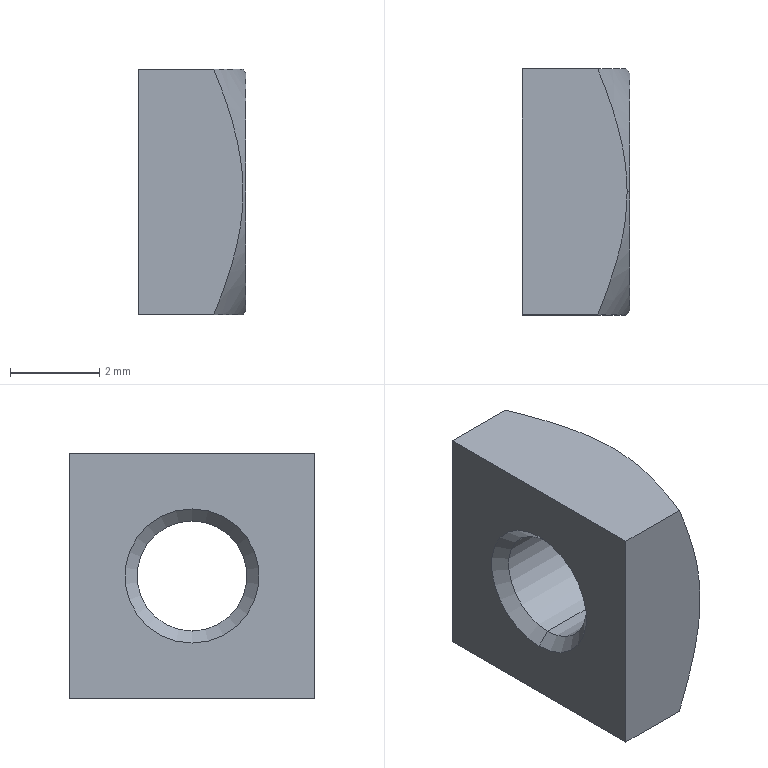Part | STEP file | Guide wheel mechanism revised.sldasm-Part-473 | 1 solid | 14 faces | box 2.4 x 5.5 x 5.5 mm | volume 58.875 mm3 | cone 6 | plane 6 | cylinder 2 | commonest cylinder face diameters 2.459 x2
STEP:
#1=CARTESIAN_POINT('',(2.129,0.,-1.229));
#2=VERTEX_POINT('',#1);
#3=CARTESIAN_POINT('',(2.129,0.,1.229));
#4=VERTEX_POINT('',#3);
#5=CARTESIAN_POINT('',(2.129,0.,0.));
#6=DIRECTION('',(-1.,0.,0.));
#7=DIRECTION('',(0.,0.,1.));
#8=AXIS2_PLACEMENT_3D('',#5,#6,#7);
#9=CIRCLE('',#8,1.229);
#10=EDGE_CURVE('',#2,#4,#9,.T.);
#11=ORIENTED_EDGE('',*,*,#10,.T.);
#12=CARTESIAN_POINT('',(2.4,0.,1.5));
#13=VERTEX_POINT('',#12);
#14=CARTESIAN_POINT('',(2.4,0.,1.5));
#15=DIRECTION('',(0.7071,0.,0.7071));
#16=VECTOR('',#15,1000.);
#17=LINE('',#14,#16);
#18=EDGE_CURVE('',#4,#13,#17,.T.);
#19=ORIENTED_EDGE('',*,*,#18,.T.);
#20=CARTESIAN_POINT('',(2.4,0.,-1.5));
#21=VERTEX_POINT('',#20);
#22=CARTESIAN_POINT('',(2.4,0.,0.));
#23=DIRECTION('',(-1.,0.,0.));
#24=DIRECTION('',(0.,0.,1.));
#25=AXIS2_PLACEMENT_3D('',#22,#23,#24);
#26=CIRCLE('',#25,1.5);
#27=EDGE_CURVE('',#21,#13,#26,.T.);
#28=ORIENTED_EDGE('',*,*,#27,.F.);
#29=CARTESIAN_POINT('',(2.4,0.,-1.5));
#30=DIRECTION('',(0.7071,0.,-0.7071));
#31=VECTOR('',#30,1000.);
#32=LINE('',#29,#31);
#33=EDGE_CURVE('',#2,#21,#32,.T.);
#34=ORIENTED_EDGE('',*,*,#33,.F.);
#35=EDGE_LOOP('',(#11,#19,#28,#34));
#36=FACE_OUTER_BOUND('',#35,.T.);
#37=CARTESIAN_POINT('',(2.4,0.,0.));
#38=DIRECTION('',(1.,0.,0.));
#39=DIRECTION('',(0.,0.,-1.));
#40=AXIS2_PLACEMENT_3D('',#37,#38,#39);
#41=CONICAL_SURFACE('',#40,1.5,0.7854);
#42=ADVANCED_FACE('',(#36),#41,.F.);
#43=ORIENTED_EDGE('',*,*,#10,.F.);
#44=CARTESIAN_POINT('',(0.2705,0.,-1.229));
#45=VERTEX_POINT('',#44);
#46=CARTESIAN_POINT('',(2.4,0.,-1.229));
#47=DIRECTION('',(-1.,0.,0.));
#48=VECTOR('',#47,1000.);
#49=LINE('',#46,#48);
#50=EDGE_CURVE('',#2,#45,#49,.T.);
#51=ORIENTED_EDGE('',*,*,#50,.T.);
#52=CARTESIAN_POINT('',(0.2705,0.,1.229));
#53=VERTEX_POINT('',#52);
#54=CARTESIAN_POINT('',(0.2705,0.,0.));
#55=DIRECTION('',(-1.,0.,0.));
#56=DIRECTION('',(0.,0.,1.));
#57=AXIS2_PLACEMENT_3D('',#54,#55,#56);
#58=CIRCLE('',#57,1.229);
#59=EDGE_CURVE('',#45,#53,#58,.T.);
#60=ORIENTED_EDGE('',*,*,#59,.T.);
#61=CARTESIAN_POINT('',(2.4,0.,1.229));
#62=DIRECTION('',(-1.,0.,0.));
#63=VECTOR('',#62,1000.);
#64=LINE('',#61,#63);
#65=EDGE_CURVE('',#4,#53,#64,.T.);
#66=ORIENTED_EDGE('',*,*,#65,.F.);
#67=EDGE_LOOP('',(#43,#51,#60,#66));
#68=FACE_OUTER_BOUND('',#67,.T.);
#69=CARTESIAN_POINT('',(2.4,0.,0.));
#70=DIRECTION('',(-1.,0.,0.));
#71=DIRECTION('',(0.,0.,1.));
#72=AXIS2_PLACEMENT_3D('',#69,#70,#71);
#73=CYLINDRICAL_SURFACE('',#72,1.229);
#74=ADVANCED_FACE('',(#68),#73,.F.);
#75=ORIENTED_EDGE('',*,*,#59,.F.);
#76=CARTESIAN_POINT('',(0.,0.,-1.5));
#77=VERTEX_POINT('',#76);
#78=CARTESIAN_POINT('',(0.2705,0.,-1.229));
#79=DIRECTION('',(-0.7071,0.,-0.7071));
#80=VECTOR('',#79,1000.);
#81=LINE('',#78,#80);
#82=EDGE_CURVE('',#45,#77,#81,.T.);
#83=ORIENTED_EDGE('',*,*,#82,.T.);
#84=CARTESIAN_POINT('',(0.,0.,1.5));
#85=VERTEX_POINT('',#84);
#86=CARTESIAN_POINT('',(0.,0.,0.));
#87=DIRECTION('',(-1.,0.,0.));
#88=DIRECTION('',(0.,0.,1.));
#89=AXIS2_PLACEMENT_3D('',#86,#87,#88);
#90=CIRCLE('',#89,1.5);
#91=EDGE_CURVE('',#77,#85,#90,.T.);
#92=ORIENTED_EDGE('',*,*,#91,.T.);
#93=CARTESIAN_POINT('',(0.2705,0.,1.229));
#94=DIRECTION('',(-0.7071,0.,0.7071));
#95=VECTOR('',#94,1000.);
#96=LINE('',#93,#95);
#97=EDGE_CURVE('',#53,#85,#96,.T.);
#98=ORIENTED_EDGE('',*,*,#97,.F.);
#99=EDGE_LOOP('',(#75,#83,#92,#98));
#100=FACE_OUTER_BOUND('',#99,.T.);
#101=CARTESIAN_POINT('',(0.2705,0.,0.));
#102=DIRECTION('',(-1.,0.,0.));
#103=DIRECTION('',(0.,0.,1.));
#104=AXIS2_PLACEMENT_3D('',#101,#102,#103);
#105=CONICAL_SURFACE('',#104,1.229,0.7854);
#106=ADVANCED_FACE('',(#100),#105,.F.);
#107=CARTESIAN_POINT('',(2.4,0.,2.65));
#108=VERTEX_POINT('',#107);
#109=CARTESIAN_POINT('',(2.4,0.,-2.65));
#110=VERTEX_POINT('',#109);
#111=CARTESIAN_POINT('',(2.4,0.,0.));
#112=DIRECTION('',(-1.,0.,0.));
#113=DIRECTION('',(0.,0.,1.));
#114=AXIS2_PLACEMENT_3D('',#111,#112,#113);
#115=CIRCLE('',#114,2.65);
#116=EDGE_CURVE('',#108,#110,#115,.T.);
#117=ORIENTED_EDGE('',*,*,#116,.T.);
#118=CARTESIAN_POINT('',(2.342,0.,-2.75));
#119=VERTEX_POINT('',#118);
#120=CARTESIAN_POINT('',(2.4,0.,-2.65));
#121=DIRECTION('',(-0.5,0.,-0.866));
#122=VECTOR('',#121,1000.);
#123=LINE('',#120,#122);
#124=EDGE_CURVE('',#110,#119,#123,.T.);
#125=ORIENTED_EDGE('',*,*,#124,.T.);
#126=CARTESIAN_POINT('',(1.685,2.75,-2.75));
#127=VERTEX_POINT('',#126);
#128=CARTESIAN_POINT('',(2.342,0.,-2.75));
#129=CARTESIAN_POINT('',(2.342,0.4777,-2.75));
#130=CARTESIAN_POINT('',(2.268,0.9433,-2.75));
#131=CARTESIAN_POINT('',(2.028,1.859,-2.75));
#132=CARTESIAN_POINT('',(1.864,2.311,-2.75));
#133=CARTESIAN_POINT('',(1.685,2.75,-2.75));
#134=B_SPLINE_CURVE_WITH_KNOTS('',3,(#128,#129,#130,#131,#132,#133),.UNSPECIFIED.,.F.,.F.,(4,2,4),(0.00576,0.007192,0.008623),.UNSPECIFIED.);
#135=EDGE_CURVE('',#119,#127,#134,.T.);
#136=ORIENTED_EDGE('',*,*,#135,.T.);
#137=CARTESIAN_POINT('',(1.685,2.75,2.75));
#138=VERTEX_POINT('',#137);
#139=CARTESIAN_POINT('',(1.685,2.75,-2.75));
#140=CARTESIAN_POINT('',(1.864,2.75,-2.309));
#141=CARTESIAN_POINT('',(2.028,2.75,-1.859));
#142=CARTESIAN_POINT('',(2.209,2.75,-1.17));
#143=CARTESIAN_POINT('',(2.258,2.75,-0.9383));
#144=CARTESIAN_POINT('',(2.325,2.75,-0.4681));
#145=CARTESIAN_POINT('',(2.343,2.75,-0.2274));
#146=CARTESIAN_POINT('',(2.341,2.75,0.4863));
#147=CARTESIAN_POINT('',(2.267,2.75,0.95));
#148=CARTESIAN_POINT('',(2.027,2.75,1.863));
#149=CARTESIAN_POINT('',(1.863,2.75,2.312));
#150=CARTESIAN_POINT('',(1.685,2.75,2.75));
#151=B_SPLINE_CURVE_WITH_KNOTS('',3,(#139,#140,#141,#142,#143,#144,#145,#146,#147,#148,#149,#150),.UNSPECIFIED.,.F.,.F.,(4,2,2,2,2,4),(0.002918,0.004344,0.005057,0.00577,0.007197,0.008623),.UNSPECIFIED.);
#152=EDGE_CURVE('',#127,#138,#151,.T.);
#153=ORIENTED_EDGE('',*,*,#152,.T.);
#154=CARTESIAN_POINT('',(2.342,0.,2.75));
#155=VERTEX_POINT('',#154);
#156=CARTESIAN_POINT('',(1.685,2.75,2.75));
#157=CARTESIAN_POINT('',(1.864,2.311,2.75));
#158=CARTESIAN_POINT('',(2.028,1.859,2.75));
#159=CARTESIAN_POINT('',(2.268,0.9433,2.75));
#160=CARTESIAN_POINT('',(2.342,0.4777,2.75));
#161=CARTESIAN_POINT('',(2.342,0.,2.75));
#162=B_SPLINE_CURVE_WITH_KNOTS('',3,(#156,#157,#158,#159,#160,#161),.UNSPECIFIED.,.F.,.F.,(4,2,4),(0.007165,0.008584,0.01),.UNSPECIFIED.);
#163=EDGE_CURVE('',#138,#155,#162,.T.);
#164=ORIENTED_EDGE('',*,*,#163,.T.);
#165=CARTESIAN_POINT('',(2.4,0.,2.65));
#166=DIRECTION('',(-0.5,0.,0.866));
#167=VECTOR('',#166,1000.);
#168=LINE('',#165,#167);
#169=EDGE_CURVE('',#108,#155,#168,.T.);
#170=ORIENTED_EDGE('',*,*,#169,.F.);
#171=EDGE_LOOP('',(#117,#125,#136,#153,#164,#170));
#172=FACE_OUTER_BOUND('',#171,.T.);
#173=CARTESIAN_POINT('',(2.4,0.,0.));
#174=DIRECTION('',(-1.,0.,0.));
#175=DIRECTION('',(0.,0.,1.));
#176=AXIS2_PLACEMENT_3D('',#173,#174,#175);
#177=CONICAL_SURFACE('',#176,2.65,1.047);
#178=ADVANCED_FACE('',(#172),#177,.T.);
#179=ORIENTED_EDGE('',*,*,#116,.F.);
#180=CARTESIAN_POINT('',(2.4,0.,0.));
#181=DIRECTION('',(-1.,0.,0.));
#182=DIRECTION('',(0.,0.,1.));
#183=AXIS2_PLACEMENT_3D('',#180,#181,#182);
#184=CIRCLE('',#183,2.65);
#185=EDGE_CURVE('',#110,#108,#184,.T.);
#186=ORIENTED_EDGE('',*,*,#185,.F.);
#187=EDGE_LOOP('',(#179,#186));
#188=FACE_OUTER_BOUND('',#187,.T.);
#189=ORIENTED_EDGE('',*,*,#27,.T.);
#190=CARTESIAN_POINT('',(2.4,0.,0.));
#191=DIRECTION('',(-1.,0.,0.));
#192=DIRECTION('',(0.,0.,1.));
#193=AXIS2_PLACEMENT_3D('',#190,#191,#192);
#194=CIRCLE('',#193,1.5);
#195=EDGE_CURVE('',#13,#21,#194,.T.);
#196=ORIENTED_EDGE('',*,*,#195,.T.);
#197=EDGE_LOOP('',(#189,#196));
#198=FACE_BOUND('',#197,.T.);
#199=CARTESIAN_POINT('',(2.4,2.65,0.));
#200=DIRECTION('',(-1.,0.,0.));
#201=DIRECTION('',(0.,0.,1.));
#202=AXIS2_PLACEMENT_3D('',#199,#200,#201);
#203=PLANE('',#202);
#204=ADVANCED_FACE('',(#188,#198),#203,.F.);
#205=CARTESIAN_POINT('',(0.,2.75,2.75));
#206=VERTEX_POINT('',#205);
#207=CARTESIAN_POINT('',(0.,-2.75,2.75));
#208=VERTEX_POINT('',#207);
#209=CARTESIAN_POINT('',(0.,2.75,2.75));
#210=DIRECTION('',(0.,-1.,0.));
#211=VECTOR('',#210,1000.);
#212=LINE('',#209,#211);
#213=EDGE_CURVE('',#206,#208,#212,.T.);
#214=ORIENTED_EDGE('',*,*,#213,.F.);
#215=CARTESIAN_POINT('',(0.,2.75,-2.75));
#216=VERTEX_POINT('',#215);
#217=CARTESIAN_POINT('',(0.,2.75,-2.75));
#218=DIRECTION('',(0.,0.,1.));
#219=VECTOR('',#218,1000.);
#220=LINE('',#217,#219);
#221=EDGE_CURVE('',#216,#206,#220,.T.);
#222=ORIENTED_EDGE('',*,*,#221,.F.);
#223=CARTESIAN_POINT('',(0.,-2.75,-2.75));
#224=VERTEX_POINT('',#223);
#225=CARTESIAN_POINT('',(0.,-2.75,-2.75));
#226=DIRECTION('',(0.,1.,0.));
#227=VECTOR('',#226,1000.);
#228=LINE('',#225,#227);
#229=EDGE_CURVE('',#224,#216,#228,.T.);
#230=ORIENTED_EDGE('',*,*,#229,.F.);
#231=CARTESIAN_POINT('',(0.,-2.75,2.75));
#232=DIRECTION('',(0.,0.,-1.));
#233=VECTOR('',#232,1000.);
#234=LINE('',#231,#233);
#235=EDGE_CURVE('',#208,#224,#234,.T.);
#236=ORIENTED_EDGE('',*,*,#235,.F.);
#237=EDGE_LOOP('',(#214,#222,#230,#236));
#238=FACE_OUTER_BOUND('',#237,.T.);
#239=CARTESIAN_POINT('',(0.,0.,0.));
#240=DIRECTION('',(-1.,0.,0.));
#241=DIRECTION('',(0.,0.,1.));
#242=AXIS2_PLACEMENT_3D('',#239,#240,#241);
#243=CIRCLE('',#242,1.5);
#244=EDGE_CURVE('',#85,#77,#243,.T.);
#245=ORIENTED_EDGE('',*,*,#244,.F.);
#246=ORIENTED_EDGE('',*,*,#91,.F.);
#247=EDGE_LOOP('',(#245,#246));
#248=FACE_BOUND('',#247,.T.);
#249=CARTESIAN_POINT('',(0.,0.,0.));
#250=DIRECTION('',(1.,0.,0.));
#251=DIRECTION('',(0.,0.,-1.));
#252=AXIS2_PLACEMENT_3D('',#249,#250,#251);
#253=PLANE('',#252);
#254=ADVANCED_FACE('',(#238,#248),#253,.F.);
#255=ORIENTED_EDGE('',*,*,#124,.F.);
#256=ORIENTED_EDGE('',*,*,#185,.T.);
#257=ORIENTED_EDGE('',*,*,#169,.T.);
#258=CARTESIAN_POINT('',(1.685,-2.75,2.75));
#259=VERTEX_POINT('',#258);
#260=CARTESIAN_POINT('',(2.342,0.,2.75));
#261=CARTESIAN_POINT('',(2.342,-0.2371,2.75));
#262=CARTESIAN_POINT('',(2.324,-0.4768,2.75));
#263=CARTESIAN_POINT('',(2.256,-0.9452,2.75));
#264=CARTESIAN_POINT('',(2.207,-1.176,2.75));
#265=CARTESIAN_POINT('',(2.027,-1.862,2.75));
#266=CARTESIAN_POINT('',(1.864,-2.311,2.75));
#267=CARTESIAN_POINT('',(1.685,-2.75,2.75));
#268=B_SPLINE_CURVE_WITH_KNOTS('',3,(#260,#261,#262,#263,#264,#265,#266,#267),.UNSPECIFIED.,.F.,.F.,(4,2,2,4),(0.01,0.01071,0.01141,0.01282),.UNSPECIFIED.);
#269=EDGE_CURVE('',#155,#259,#268,.T.);
#270=ORIENTED_EDGE('',*,*,#269,.T.);
#271=CARTESIAN_POINT('',(1.685,-2.75,-2.75));
#272=VERTEX_POINT('',#271);
#273=CARTESIAN_POINT('',(1.685,-2.75,2.75));
#274=CARTESIAN_POINT('',(1.863,-2.75,2.312));
#275=CARTESIAN_POINT('',(2.027,-2.75,1.863));
#276=CARTESIAN_POINT('',(2.267,-2.75,0.95));
#277=CARTESIAN_POINT('',(2.341,-2.75,0.4863));
#278=CARTESIAN_POINT('',(2.343,-2.75,-0.2274));
#279=CARTESIAN_POINT('',(2.325,-2.75,-0.4681));
#280=CARTESIAN_POINT('',(2.258,-2.75,-0.9383));
#281=CARTESIAN_POINT('',(2.209,-2.75,-1.17));
#282=CARTESIAN_POINT('',(2.028,-2.75,-1.859));
#283=CARTESIAN_POINT('',(1.864,-2.75,-2.309));
#284=CARTESIAN_POINT('',(1.685,-2.75,-2.75));
#285=B_SPLINE_CURVE_WITH_KNOTS('',3,(#273,#274,#275,#276,#277,#278,#279,#280,#281,#282,#283,#284),.UNSPECIFIED.,.F.,.F.,(4,2,2,2,2,4),(0.007165,0.008579,0.009994,0.0107,0.01141,0.01282),.UNSPECIFIED.);
#286=EDGE_CURVE('',#259,#272,#285,.T.);
#287=ORIENTED_EDGE('',*,*,#286,.T.);
#288=CARTESIAN_POINT('',(1.685,-2.75,-2.75));
#289=CARTESIAN_POINT('',(1.864,-2.311,-2.75));
#290=CARTESIAN_POINT('',(2.027,-1.862,-2.75));
#291=CARTESIAN_POINT('',(2.207,-1.176,-2.75));
#292=CARTESIAN_POINT('',(2.256,-0.9452,-2.75));
#293=CARTESIAN_POINT('',(2.324,-0.4768,-2.75));
#294=CARTESIAN_POINT('',(2.342,-0.2371,-2.75));
#295=CARTESIAN_POINT('',(2.342,0.,-2.75));
#296=B_SPLINE_CURVE_WITH_KNOTS('',3,(#288,#289,#290,#291,#292,#293,#294,#295),.UNSPECIFIED.,.F.,.F.,(4,2,2,4),(0.002918,0.004339,0.005049,0.00576),.UNSPECIFIED.);
#297=EDGE_CURVE('',#272,#119,#296,.T.);
#298=ORIENTED_EDGE('',*,*,#297,.T.);
#299=EDGE_LOOP('',(#255,#256,#257,#270,#287,#298));
#300=FACE_OUTER_BOUND('',#299,.T.);
#301=CARTESIAN_POINT('',(2.4,0.,0.));
#302=DIRECTION('',(-1.,0.,0.));
#303=DIRECTION('',(0.,0.,1.));
#304=AXIS2_PLACEMENT_3D('',#301,#302,#303);
#305=CONICAL_SURFACE('',#304,2.65,1.047);
#306=ADVANCED_FACE('',(#300),#305,.T.);
#307=CARTESIAN_POINT('',(6.,2.75,-2.75));
#308=DIRECTION('',(-1.,0.,0.));
#309=VECTOR('',#308,1000.);
#310=LINE('',#307,#309);
#311=EDGE_CURVE('',#127,#216,#310,.T.);
#312=ORIENTED_EDGE('',*,*,#311,.T.);
#313=ORIENTED_EDGE('',*,*,#221,.T.);
#314=CARTESIAN_POINT('',(6.,2.75,2.75));
#315=DIRECTION('',(-1.,0.,0.));
#316=VECTOR('',#315,1000.);
#317=LINE('',#314,#316);
#318=EDGE_CURVE('',#138,#206,#317,.T.);
#319=ORIENTED_EDGE('',*,*,#318,.F.);
#320=ORIENTED_EDGE('',*,*,#152,.F.);
#321=EDGE_LOOP('',(#312,#313,#319,#320));
#322=FACE_OUTER_BOUND('',#321,.T.);
#323=CARTESIAN_POINT('',(6.,2.75,-2.75));
#324=DIRECTION('',(0.,-1.,0.));
#325=DIRECTION('',(0.,0.,-1.));
#326=AXIS2_PLACEMENT_3D('',#323,#324,#325);
#327=PLANE('',#326);
#328=ADVANCED_FACE('',(#322),#327,.F.);
#329=ORIENTED_EDGE('',*,*,#318,.T.);
#330=ORIENTED_EDGE('',*,*,#213,.T.);
#331=CARTESIAN_POINT('',(6.,-2.75,2.75));
#332=DIRECTION('',(-1.,0.,0.));
#333=VECTOR('',#332,1000.);
#334=LINE('',#331,#333);
#335=EDGE_CURVE('',#259,#208,#334,.T.);
#336=ORIENTED_EDGE('',*,*,#335,.F.);
#337=ORIENTED_EDGE('',*,*,#269,.F.);
#338=ORIENTED_EDGE('',*,*,#163,.F.);
#339=EDGE_LOOP('',(#329,#330,#336,#337,#338));
#340=FACE_OUTER_BOUND('',#339,.T.);
#341=CARTESIAN_POINT('',(6.,2.75,2.75));
#342=DIRECTION('',(0.,0.,-1.));
#343=DIRECTION('',(-1.,0.,0.));
#344=AXIS2_PLACEMENT_3D('',#341,#342,#343);
#345=PLANE('',#344);
#346=ADVANCED_FACE('',(#340),#345,.F.);
#347=ORIENTED_EDGE('',*,*,#335,.T.);
#348=ORIENTED_EDGE('',*,*,#235,.T.);
#349=CARTESIAN_POINT('',(6.,-2.75,-2.75));
#350=DIRECTION('',(-1.,0.,0.));
#351=VECTOR('',#350,1000.);
#352=LINE('',#349,#351);
#353=EDGE_CURVE('',#272,#224,#352,.T.);
#354=ORIENTED_EDGE('',*,*,#353,.F.);
#355=ORIENTED_EDGE('',*,*,#286,.F.);
#356=EDGE_LOOP('',(#347,#348,#354,#355));
#357=FACE_OUTER_BOUND('',#356,.T.);
#358=CARTESIAN_POINT('',(6.,-2.75,2.75));
#359=DIRECTION('',(0.,1.,0.));
#360=DIRECTION('',(0.,0.,1.));
#361=AXIS2_PLACEMENT_3D('',#358,#359,#360);
#362=PLANE('',#361);
#363=ADVANCED_FACE('',(#357),#362,.F.);
#364=ORIENTED_EDGE('',*,*,#353,.T.);
#365=ORIENTED_EDGE('',*,*,#229,.T.);
#366=ORIENTED_EDGE('',*,*,#311,.F.);
#367=ORIENTED_EDGE('',*,*,#135,.F.);
#368=ORIENTED_EDGE('',*,*,#297,.F.);
#369=EDGE_LOOP('',(#364,#365,#366,#367,#368));
#370=FACE_OUTER_BOUND('',#369,.T.);
#371=CARTESIAN_POINT('',(6.,-2.75,-2.75));
#372=DIRECTION('',(0.,0.,1.));
#373=DIRECTION('',(1.,0.,0.));
#374=AXIS2_PLACEMENT_3D('',#371,#372,#373);
#375=PLANE('',#374);
#376=ADVANCED_FACE('',(#370),#375,.F.);
#377=ORIENTED_EDGE('',*,*,#82,.F.);
#378=CARTESIAN_POINT('',(0.2705,0.,0.));
#379=DIRECTION('',(-1.,0.,0.));
#380=DIRECTION('',(0.,0.,1.));
#381=AXIS2_PLACEMENT_3D('',#378,#379,#380);
#382=CIRCLE('',#381,1.229);
#383=EDGE_CURVE('',#53,#45,#382,.T.);
#384=ORIENTED_EDGE('',*,*,#383,.F.);
#385=ORIENTED_EDGE('',*,*,#97,.T.);
#386=ORIENTED_EDGE('',*,*,#244,.T.);
#387=EDGE_LOOP('',(#377,#384,#385,#386));
#388=FACE_OUTER_BOUND('',#387,.T.);
#389=CARTESIAN_POINT('',(0.2705,0.,0.));
#390=DIRECTION('',(-1.,0.,0.));
#391=DIRECTION('',(0.,0.,1.));
#392=AXIS2_PLACEMENT_3D('',#389,#390,#391);
#393=CONICAL_SURFACE('',#392,1.229,0.7854);
#394=ADVANCED_FACE('',(#388),#393,.F.);
#395=ORIENTED_EDGE('',*,*,#50,.F.);
#396=CARTESIAN_POINT('',(2.129,0.,0.));
#397=DIRECTION('',(-1.,0.,0.));
#398=DIRECTION('',(0.,0.,1.));
#399=AXIS2_PLACEMENT_3D('',#396,#397,#398);
#400=CIRCLE('',#399,1.229);
#401=EDGE_CURVE('',#4,#2,#400,.T.);
#402=ORIENTED_EDGE('',*,*,#401,.F.);
#403=ORIENTED_EDGE('',*,*,#65,.T.);
#404=ORIENTED_EDGE('',*,*,#383,.T.);
#405=EDGE_LOOP('',(#395,#402,#403,#404));
#406=FACE_OUTER_BOUND('',#405,.T.);
#407=CARTESIAN_POINT('',(2.4,0.,0.));
#408=DIRECTION('',(-1.,0.,0.));
#409=DIRECTION('',(0.,0.,1.));
#410=AXIS2_PLACEMENT_3D('',#407,#408,#409);
#411=CYLINDRICAL_SURFACE('',#410,1.229);
#412=ADVANCED_FACE('',(#406),#411,.F.);
#413=ORIENTED_EDGE('',*,*,#18,.F.);
#414=ORIENTED_EDGE('',*,*,#401,.T.);
#415=ORIENTED_EDGE('',*,*,#33,.T.);
#416=ORIENTED_EDGE('',*,*,#195,.F.);
#417=EDGE_LOOP('',(#413,#414,#415,#416));
#418=FACE_OUTER_BOUND('',#417,.T.);
#419=CARTESIAN_POINT('',(2.4,0.,0.));
#420=DIRECTION('',(1.,0.,0.));
#421=DIRECTION('',(0.,0.,-1.));
#422=AXIS2_PLACEMENT_3D('',#419,#420,#421);
#423=CONICAL_SURFACE('',#422,1.5,0.7854);
#424=ADVANCED_FACE('',(#418),#423,.F.);
#425=CLOSED_SHELL('',(#42,#74,#106,#178,#204,#254,#306,#328,#346,#363,#376,#394,#412,#424));
#426=MANIFOLD_SOLID_BREP('',#425);
#427=CARTESIAN_POINT('',(0.,0.,0.));
#428=DIRECTION('',(0.,0.,1.));
#429=DIRECTION('',(1.,0.,0.));
#430=AXIS2_PLACEMENT_3D('',#427,#428,#429);
#431=(LENGTH_UNIT()NAMED_UNIT(*)SI_UNIT(.MILLI.,.METRE.));
#432=UNCERTAINTY_MEASURE_WITH_UNIT(LENGTH_MEASURE(0.00001),#431,'','');
#433=(NAMED_UNIT(*)PLANE_ANGLE_UNIT()SI_UNIT($,.RADIAN.));
#434=(NAMED_UNIT(*)SI_UNIT($,.STERADIAN.)SOLID_ANGLE_UNIT());
#435=(GEOMETRIC_REPRESENTATION_CONTEXT(3)GLOBAL_UNCERTAINTY_ASSIGNED_CONTEXT((#432))GLOBAL_UNIT_ASSIGNED_CONTEXT((#431,#433,#434))REPRESENTATION_CONTEXT('',''));
#436=ADVANCED_BREP_SHAPE_REPRESENTATION('',(#426,#430),#435);